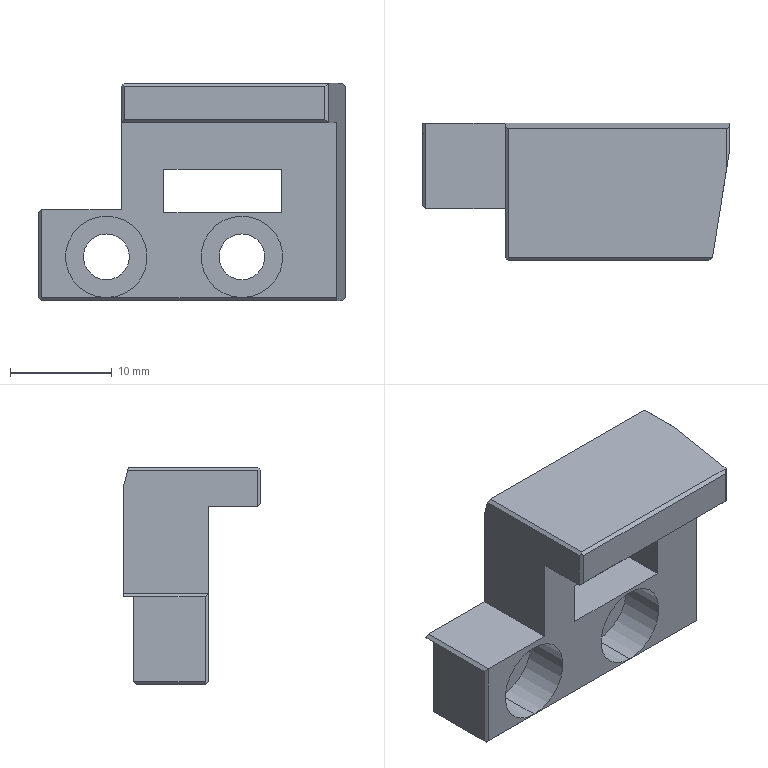Part | NX | 1 solid | 41 faces | box 30.1 x 13.5 x 21.378 mm | volume 3668 mm3 | plane 33 | cylinder 8 | commonest cylinder face diameters 4.5 x4 8 x4
STEP:
#1=CARTESIAN_POINT('',(-190.3,206.36,-59.));
#2=VERTEX_POINT('',#1);
#3=CARTESIAN_POINT('',(-219.8,206.36,-59.));
#4=VERTEX_POINT('',#3);
#5=CARTESIAN_POINT('',(-205.05,206.36,-59.));
#6=DIRECTION('',(-1.,0.,0.));
#7=VECTOR('',#6,1000.);
#8=LINE('',#5,#7);
#9=EDGE_CURVE('',#2,#4,#8,.T.);
#10=ORIENTED_EDGE('',*,*,#9,.F.);
#11=CARTESIAN_POINT('',(-190.3,202.995,-59.));
#12=VERTEX_POINT('',#11);
#13=CARTESIAN_POINT('',(-190.3,205.774,-59.));
#14=DIRECTION('',(0.,-1.,0.));
#15=VECTOR('',#14,1000.);
#16=LINE('',#13,#15);
#17=EDGE_CURVE('',#2,#12,#16,.T.);
#18=ORIENTED_EDGE('',*,*,#17,.T.);
#19=CARTESIAN_POINT('',(-190.838,199.6,-59.));
#20=VERTEX_POINT('',#19);
#21=CARTESIAN_POINT('',(-190.024,204.737,-59.));
#22=DIRECTION('',(0.1564,0.9877,0.));
#23=VECTOR('',#22,1000.);
#24=LINE('',#21,#23);
#25=EDGE_CURVE('',#20,#12,#24,.T.);
#26=ORIENTED_EDGE('',*,*,#25,.F.);
#27=CARTESIAN_POINT('',(-219.8,199.6,-59.));
#28=VERTEX_POINT('',#27);
#29=CARTESIAN_POINT('',(-205.493,199.6,-59.));
#30=DIRECTION('',(-1.,0.,0.));
#31=VECTOR('',#30,1000.);
#32=LINE('',#29,#31);
#33=EDGE_CURVE('',#20,#28,#32,.T.);
#34=ORIENTED_EDGE('',*,*,#33,.T.);
#35=CARTESIAN_POINT('',(-219.8,202.98,-59.));
#36=DIRECTION('',(0.,1.,0.));
#37=VECTOR('',#36,1000.);
#38=LINE('',#35,#37);
#39=EDGE_CURVE('',#28,#4,#38,.T.);
#40=ORIENTED_EDGE('',*,*,#39,.T.);
#41=EDGE_LOOP('',(#10,#18,#26,#34,#40));
#42=FACE_BOUND('',#41,.T.);
#43=CARTESIAN_POINT('',(-190.,199.3,-59.));
#44=DIRECTION('',(0.,0.,-1.));
#45=DIRECTION('',(0.,-1.,0.));
#46=AXIS2_PLACEMENT_3D('',#43,#44,#45);
#47=PLANE('',#46);
#48=ADVANCED_FACE('',(#42),#47,.T.);
#49=CARTESIAN_POINT('',(-211.7,194.16,-41.2));
#50=VERTEX_POINT('',#49);
#51=CARTESIAN_POINT('',(-191.999,194.16,-41.2));
#52=VERTEX_POINT('',#51);
#53=CARTESIAN_POINT('',(-201.85,194.16,-41.2));
#54=DIRECTION('',(1.,0.,0.));
#55=VECTOR('',#54,1000.);
#56=LINE('',#53,#55);
#57=EDGE_CURVE('',#50,#52,#56,.T.);
#58=ORIENTED_EDGE('',*,*,#57,.T.);
#59=CARTESIAN_POINT('',(-191.999,194.16,-37.922));
#60=VERTEX_POINT('',#59);
#61=CARTESIAN_POINT('',(-191.999,194.16,-39.561));
#62=DIRECTION('',(0.,0.,1.));
#63=VECTOR('',#62,1000.);
#64=LINE('',#61,#63);
#65=EDGE_CURVE('',#52,#60,#64,.T.);
#66=ORIENTED_EDGE('',*,*,#65,.T.);
#67=CARTESIAN_POINT('',(-211.7,194.16,-37.922));
#68=VERTEX_POINT('',#67);
#69=CARTESIAN_POINT('',(-201.85,194.16,-37.922));
#70=DIRECTION('',(1.,0.,0.));
#71=VECTOR('',#70,1000.);
#72=LINE('',#69,#71);
#73=EDGE_CURVE('',#68,#60,#72,.T.);
#74=ORIENTED_EDGE('',*,*,#73,.F.);
#75=CARTESIAN_POINT('',(-211.7,194.16,-39.561));
#76=DIRECTION('',(0.,0.,1.));
#77=VECTOR('',#76,1000.);
#78=LINE('',#75,#77);
#79=EDGE_CURVE('',#50,#68,#78,.T.);
#80=ORIENTED_EDGE('',*,*,#79,.F.);
#81=EDGE_LOOP('',(#58,#66,#74,#80));
#82=FACE_BOUND('',#81,.T.);
#83=CARTESIAN_POINT('',(-190.,194.16,-37.622));
#84=DIRECTION('',(0.,-1.,0.));
#85=DIRECTION('',(-1.,0.,0.));
#86=AXIS2_PLACEMENT_3D('',#83,#84,#85);
#87=PLANE('',#86);
#88=ADVANCED_FACE('',(#82),#87,.T.);
#89=CARTESIAN_POINT('',(-190.3,207.16,-37.622));
#90=VERTEX_POINT('',#89);
#91=CARTESIAN_POINT('',(-211.7,207.16,-37.622));
#92=VERTEX_POINT('',#91);
#93=CARTESIAN_POINT('',(-201.,207.16,-37.622));
#94=DIRECTION('',(-1.,0.,0.));
#95=VECTOR('',#94,1000.);
#96=LINE('',#93,#95);
#97=EDGE_CURVE('',#90,#92,#96,.T.);
#98=ORIENTED_EDGE('',*,*,#97,.T.);
#99=CARTESIAN_POINT('',(-211.7,194.46,-37.622));
#100=VERTEX_POINT('',#99);
#101=CARTESIAN_POINT('',(-211.7,204.737,-37.622));
#102=DIRECTION('',(0.,1.,0.));
#103=VECTOR('',#102,1000.);
#104=LINE('',#101,#103);
#105=EDGE_CURVE('',#100,#92,#104,.T.);
#106=ORIENTED_EDGE('',*,*,#105,.F.);
#107=CARTESIAN_POINT('',(-191.652,194.46,-37.622));
#108=VERTEX_POINT('',#107);
#109=CARTESIAN_POINT('',(-201.85,194.46,-37.622));
#110=DIRECTION('',(1.,0.,0.));
#111=VECTOR('',#110,1000.);
#112=LINE('',#109,#111);
#113=EDGE_CURVE('',#100,#108,#112,.T.);
#114=ORIENTED_EDGE('',*,*,#113,.T.);
#115=CARTESIAN_POINT('',(-190.3,202.995,-37.622));
#116=VERTEX_POINT('',#115);
#117=CARTESIAN_POINT('',(-190.024,204.737,-37.622));
#118=DIRECTION('',(-0.1564,-0.9877,0.));
#119=VECTOR('',#118,1000.);
#120=LINE('',#117,#119);
#121=EDGE_CURVE('',#116,#108,#120,.T.);
#122=ORIENTED_EDGE('',*,*,#121,.F.);
#123=CARTESIAN_POINT('',(-190.3,206.274,-37.622));
#124=DIRECTION('',(0.,-1.,0.));
#125=VECTOR('',#124,1000.);
#126=LINE('',#123,#125);
#127=EDGE_CURVE('',#90,#116,#126,.T.);
#128=ORIENTED_EDGE('',*,*,#127,.F.);
#129=EDGE_LOOP('',(#98,#106,#114,#122,#128));
#130=FACE_BOUND('',#129,.T.);
#131=CARTESIAN_POINT('',(-190.,207.9,-37.622));
#132=DIRECTION('',(0.,0.,1.));
#133=DIRECTION('',(1.,0.,0.));
#134=AXIS2_PLACEMENT_3D('',#131,#132,#133);
#135=PLANE('',#134);
#136=ADVANCED_FACE('',(#130),#135,.T.);
#137=CARTESIAN_POINT('',(-196.3,206.66,-50.35));
#138=VERTEX_POINT('',#137);
#139=CARTESIAN_POINT('',(-196.3,199.3,-50.35));
#140=VERTEX_POINT('',#139);
#141=CARTESIAN_POINT('',(-196.3,204.737,-50.35));
#142=DIRECTION('',(0.,-1.,0.));
#143=VECTOR('',#142,1000.);
#144=LINE('',#141,#143);
#145=EDGE_CURVE('',#138,#140,#144,.T.);
#146=ORIENTED_EDGE('',*,*,#145,.F.);
#147=CARTESIAN_POINT('',(-207.8,206.66,-50.35));
#148=VERTEX_POINT('',#147);
#149=CARTESIAN_POINT('',(-190.,206.66,-50.35));
#150=DIRECTION('',(-1.,0.,0.));
#151=VECTOR('',#150,1000.);
#152=LINE('',#149,#151);
#153=EDGE_CURVE('',#138,#148,#152,.T.);
#154=ORIENTED_EDGE('',*,*,#153,.T.);
#155=CARTESIAN_POINT('',(-207.8,199.3,-50.35));
#156=VERTEX_POINT('',#155);
#157=CARTESIAN_POINT('',(-207.8,204.737,-50.35));
#158=DIRECTION('',(0.,1.,0.));
#159=VECTOR('',#158,1000.);
#160=LINE('',#157,#159);
#161=EDGE_CURVE('',#156,#148,#160,.T.);
#162=ORIENTED_EDGE('',*,*,#161,.F.);
#163=CARTESIAN_POINT('',(-190.,199.3,-50.35));
#164=DIRECTION('',(-1.,0.,0.));
#165=VECTOR('',#164,1000.);
#166=LINE('',#163,#165);
#167=EDGE_CURVE('',#140,#156,#166,.T.);
#168=ORIENTED_EDGE('',*,*,#167,.F.);
#169=EDGE_LOOP('',(#146,#154,#162,#168));
#170=FACE_BOUND('',#169,.T.);
#171=CARTESIAN_POINT('',(-206.8,198.44,-50.35));
#172=DIRECTION('',(0.,0.,-1.));
#173=DIRECTION('',(0.,-1.,0.));
#174=AXIS2_PLACEMENT_3D('',#171,#172,#173);
#175=PLANE('',#174);
#176=ADVANCED_FACE('',(#170),#175,.F.);
#177=CARTESIAN_POINT('',(-212.,207.66,-50.05));
#178=VERTEX_POINT('',#177);
#179=CARTESIAN_POINT('',(-219.8,207.66,-50.05));
#180=VERTEX_POINT('',#179);
#181=CARTESIAN_POINT('',(-190.,207.66,-50.05));
#182=DIRECTION('',(-1.,0.,0.));
#183=VECTOR('',#182,1000.);
#184=LINE('',#181,#183);
#185=EDGE_CURVE('',#178,#180,#184,.T.);
#186=ORIENTED_EDGE('',*,*,#185,.T.);
#187=CARTESIAN_POINT('',(-219.8,199.3,-50.05));
#188=VERTEX_POINT('',#187);
#189=CARTESIAN_POINT('',(-219.8,203.48,-50.05));
#190=DIRECTION('',(0.,-1.,0.));
#191=VECTOR('',#190,1000.);
#192=LINE('',#189,#191);
#193=EDGE_CURVE('',#180,#188,#192,.T.);
#194=ORIENTED_EDGE('',*,*,#193,.T.);
#195=CARTESIAN_POINT('',(-212.,199.3,-50.05));
#196=VERTEX_POINT('',#195);
#197=CARTESIAN_POINT('',(-190.,199.3,-50.05));
#198=DIRECTION('',(1.,0.,0.));
#199=VECTOR('',#198,1000.);
#200=LINE('',#197,#199);
#201=EDGE_CURVE('',#188,#196,#200,.T.);
#202=ORIENTED_EDGE('',*,*,#201,.T.);
#203=CARTESIAN_POINT('',(-212.,204.737,-50.05));
#204=DIRECTION('',(0.,-1.,0.));
#205=VECTOR('',#204,1000.);
#206=LINE('',#203,#205);
#207=EDGE_CURVE('',#178,#196,#206,.T.);
#208=ORIENTED_EDGE('',*,*,#207,.F.);
#209=EDGE_LOOP('',(#186,#194,#202,#208));
#210=FACE_BOUND('',#209,.T.);
#211=CARTESIAN_POINT('',(-216.1,198.44,-50.05));
#212=DIRECTION('',(0.,0.,-1.));
#213=DIRECTION('',(0.,-1.,0.));
#214=AXIS2_PLACEMENT_3D('',#211,#212,#213);
#215=PLANE('',#214);
#216=ADVANCED_FACE('',(#210),#215,.F.);
#217=CARTESIAN_POINT('',(-212.,194.46,-41.5));
#218=VERTEX_POINT('',#217);
#219=CARTESIAN_POINT('',(-212.,194.46,-37.922));
#220=VERTEX_POINT('',#219);
#221=CARTESIAN_POINT('',(-212.,194.46,-39.561));
#222=DIRECTION('',(0.,0.,1.));
#223=VECTOR('',#222,1000.);
#224=LINE('',#221,#223);
#225=EDGE_CURVE('',#218,#220,#224,.T.);
#226=ORIENTED_EDGE('',*,*,#225,.T.);
#227=CARTESIAN_POINT('',(-212.,207.235,-37.922));
#228=VERTEX_POINT('',#227);
#229=CARTESIAN_POINT('',(-212.,204.737,-37.922));
#230=DIRECTION('',(0.,1.,0.));
#231=VECTOR('',#230,1000.);
#232=LINE('',#229,#231);
#233=EDGE_CURVE('',#220,#228,#232,.T.);
#234=ORIENTED_EDGE('',*,*,#233,.T.);
#235=CARTESIAN_POINT('',(-212.,207.66,-39.622));
#236=VERTEX_POINT('',#235);
#237=CARTESIAN_POINT('',(-212.,208.682,-43.71));
#238=DIRECTION('',(0.,0.2425,-0.9701));
#239=VECTOR('',#238,1000.);
#240=LINE('',#237,#239);
#241=EDGE_CURVE('',#228,#236,#240,.T.);
#242=ORIENTED_EDGE('',*,*,#241,.T.);
#243=CARTESIAN_POINT('',(-212.,207.66,-43.71));
#244=DIRECTION('',(0.,0.,1.));
#245=VECTOR('',#244,1000.);
#246=LINE('',#243,#245);
#247=EDGE_CURVE('',#178,#236,#246,.T.);
#248=ORIENTED_EDGE('',*,*,#247,.F.);
#249=ORIENTED_EDGE('',*,*,#207,.T.);
#250=CARTESIAN_POINT('',(-212.,199.3,-41.5));
#251=VERTEX_POINT('',#250);
#252=CARTESIAN_POINT('',(-212.,199.3,-43.71));
#253=DIRECTION('',(0.,0.,1.));
#254=VECTOR('',#253,1000.);
#255=LINE('',#252,#254);
#256=EDGE_CURVE('',#196,#251,#255,.T.);
#257=ORIENTED_EDGE('',*,*,#256,.T.);
#258=CARTESIAN_POINT('',(-212.,204.737,-41.5));
#259=DIRECTION('',(0.,1.,0.));
#260=VECTOR('',#259,1000.);
#261=LINE('',#258,#260);
#262=EDGE_CURVE('',#218,#251,#261,.T.);
#263=ORIENTED_EDGE('',*,*,#262,.F.);
#264=EDGE_LOOP('',(#226,#234,#242,#248,#249,#257,#263));
#265=FACE_BOUND('',#264,.T.);
#266=CARTESIAN_POINT('',(-212.,198.44,-46.8));
#267=DIRECTION('',(1.,0.,0.));
#268=DIRECTION('',(0.,-1.,0.));
#269=AXIS2_PLACEMENT_3D('',#266,#267,#268);
#270=PLANE('',#269);
#271=ADVANCED_FACE('',(#265),#270,.F.);
#272=ORIENTED_EDGE('',*,*,#225,.F.);
#273=CARTESIAN_POINT('',(-190.,172.46,-19.5));
#274=DIRECTION('',(0.5774,-0.5774,0.5774));
#275=VECTOR('',#274,1000.);
#276=LINE('',#273,#275);
#277=EDGE_CURVE('',#218,#50,#276,.T.);
#278=ORIENTED_EDGE('',*,*,#277,.T.);
#279=ORIENTED_EDGE('',*,*,#79,.T.);
#280=CARTESIAN_POINT('',(-211.85,194.31,-37.772));
#281=VERTEX_POINT('',#280);
#282=CARTESIAN_POINT('',(-190.,172.46,-59.622));
#283=DIRECTION('',(0.5774,-0.5774,-0.5774));
#284=VECTOR('',#283,1000.);
#285=LINE('',#282,#284);
#286=EDGE_CURVE('',#281,#68,#285,.T.);
#287=ORIENTED_EDGE('',*,*,#286,.F.);
#288=CARTESIAN_POINT('',(-190.,172.46,-15.922));
#289=DIRECTION('',(0.5774,-0.5774,0.5774));
#290=VECTOR('',#289,1000.);
#291=LINE('',#288,#290);
#292=EDGE_CURVE('',#220,#281,#291,.T.);
#293=ORIENTED_EDGE('',*,*,#292,.F.);
#294=EDGE_LOOP('',(#272,#278,#279,#287,#293));
#295=FACE_BOUND('',#294,.T.);
#296=CARTESIAN_POINT('',(-211.85,194.31,-39.561));
#297=DIRECTION('',(-0.7071,-0.7071,0.));
#298=DIRECTION('',(-0.7071,0.7071,0.));
#299=AXIS2_PLACEMENT_3D('',#296,#297,#298);
#300=PLANE('',#299);
#301=ADVANCED_FACE('',(#295),#300,.T.);
#302=CARTESIAN_POINT('',(-196.3,207.66,-50.35));
#303=VERTEX_POINT('',#302);
#304=CARTESIAN_POINT('',(-196.3,204.737,-50.35));
#305=DIRECTION('',(0.,1.,0.));
#306=VECTOR('',#305,1000.);
#307=LINE('',#304,#306);
#308=EDGE_CURVE('',#138,#303,#307,.T.);
#309=ORIENTED_EDGE('',*,*,#308,.F.);
#310=ORIENTED_EDGE('',*,*,#145,.T.);
#311=CARTESIAN_POINT('',(-196.3,199.3,-46.1));
#312=VERTEX_POINT('',#311);
#313=CARTESIAN_POINT('',(-196.3,199.3,-43.71));
#314=DIRECTION('',(0.,0.,1.));
#315=VECTOR('',#314,1000.);
#316=LINE('',#313,#315);
#317=EDGE_CURVE('',#140,#312,#316,.T.);
#318=ORIENTED_EDGE('',*,*,#317,.T.);
#319=CARTESIAN_POINT('',(-196.3,207.66,-46.1));
#320=VERTEX_POINT('',#319);
#321=CARTESIAN_POINT('',(-196.3,204.737,-46.1));
#322=DIRECTION('',(0.,1.,0.));
#323=VECTOR('',#322,1000.);
#324=LINE('',#321,#323);
#325=EDGE_CURVE('',#312,#320,#324,.T.);
#326=ORIENTED_EDGE('',*,*,#325,.T.);
#327=CARTESIAN_POINT('',(-196.3,207.66,-43.71));
#328=DIRECTION('',(0.,0.,-1.));
#329=VECTOR('',#328,1000.);
#330=LINE('',#327,#329);
#331=EDGE_CURVE('',#320,#303,#330,.T.);
#332=ORIENTED_EDGE('',*,*,#331,.T.);
#333=EDGE_LOOP('',(#309,#310,#318,#326,#332));
#334=FACE_BOUND('',#333,.T.);
#335=CARTESIAN_POINT('',(-196.3,198.44,-50.35));
#336=DIRECTION('',(1.,0.,0.));
#337=DIRECTION('',(0.,-1.,0.));
#338=AXIS2_PLACEMENT_3D('',#335,#336,#337);
#339=PLANE('',#338);
#340=ADVANCED_FACE('',(#334),#339,.F.);
#341=CARTESIAN_POINT('',(-207.8,199.3,-46.1));
#342=VERTEX_POINT('',#341);
#343=CARTESIAN_POINT('',(-207.8,199.3,-43.71));
#344=DIRECTION('',(0.,0.,1.));
#345=VECTOR('',#344,1000.);
#346=LINE('',#343,#345);
#347=EDGE_CURVE('',#156,#342,#346,.T.);
#348=ORIENTED_EDGE('',*,*,#347,.F.);
#349=ORIENTED_EDGE('',*,*,#161,.T.);
#350=CARTESIAN_POINT('',(-207.8,207.66,-50.35));
#351=VERTEX_POINT('',#350);
#352=CARTESIAN_POINT('',(-207.8,204.737,-50.35));
#353=DIRECTION('',(0.,1.,0.));
#354=VECTOR('',#353,1000.);
#355=LINE('',#352,#354);
#356=EDGE_CURVE('',#148,#351,#355,.T.);
#357=ORIENTED_EDGE('',*,*,#356,.T.);
#358=CARTESIAN_POINT('',(-207.8,207.66,-46.1));
#359=VERTEX_POINT('',#358);
#360=CARTESIAN_POINT('',(-207.8,207.66,-43.71));
#361=DIRECTION('',(0.,0.,1.));
#362=VECTOR('',#361,1000.);
#363=LINE('',#360,#362);
#364=EDGE_CURVE('',#351,#359,#363,.T.);
#365=ORIENTED_EDGE('',*,*,#364,.T.);
#366=CARTESIAN_POINT('',(-207.8,204.737,-46.1));
#367=DIRECTION('',(0.,1.,0.));
#368=VECTOR('',#367,1000.);
#369=LINE('',#366,#368);
#370=EDGE_CURVE('',#342,#359,#369,.T.);
#371=ORIENTED_EDGE('',*,*,#370,.F.);
#372=EDGE_LOOP('',(#348,#349,#357,#365,#371));
#373=FACE_BOUND('',#372,.T.);
#374=CARTESIAN_POINT('',(-207.8,198.44,-47.1));
#375=DIRECTION('',(-1.,0.,0.));
#376=DIRECTION('',(0.,0.,1.));
#377=AXIS2_PLACEMENT_3D('',#374,#375,#376);
#378=PLANE('',#377);
#379=ADVANCED_FACE('',(#373),#378,.F.);
#380=ORIENTED_EDGE('',*,*,#247,.T.);
#381=CARTESIAN_POINT('',(-190.,207.66,-39.622));
#382=VERTEX_POINT('',#381);
#383=CARTESIAN_POINT('',(-201.,207.66,-39.622));
#384=DIRECTION('',(-1.,0.,0.));
#385=VECTOR('',#384,1000.);
#386=LINE('',#383,#385);
#387=EDGE_CURVE('',#382,#236,#386,.T.);
#388=ORIENTED_EDGE('',*,*,#387,.F.);
#389=CARTESIAN_POINT('',(-190.,207.66,-50.35));
#390=VERTEX_POINT('',#389);
#391=CARTESIAN_POINT('',(-190.,207.66,-43.71));
#392=DIRECTION('',(0.,0.,-1.));
#393=VECTOR('',#392,1000.);
#394=LINE('',#391,#393);
#395=EDGE_CURVE('',#382,#390,#394,.T.);
#396=ORIENTED_EDGE('',*,*,#395,.T.);
#397=CARTESIAN_POINT('',(-190.,207.66,-50.35));
#398=DIRECTION('',(1.,0.,0.));
#399=VECTOR('',#398,1000.);
#400=LINE('',#397,#399);
#401=EDGE_CURVE('',#303,#390,#400,.T.);
#402=ORIENTED_EDGE('',*,*,#401,.F.);
#403=ORIENTED_EDGE('',*,*,#331,.F.);
#404=CARTESIAN_POINT('',(-190.,207.66,-46.1));
#405=DIRECTION('',(-1.,0.,0.));
#406=VECTOR('',#405,1000.);
#407=LINE('',#404,#406);
#408=EDGE_CURVE('',#320,#359,#407,.T.);
#409=ORIENTED_EDGE('',*,*,#408,.T.);
#410=ORIENTED_EDGE('',*,*,#364,.F.);
#411=CARTESIAN_POINT('',(-220.1,207.66,-50.35));
#412=VERTEX_POINT('',#411);
#413=CARTESIAN_POINT('',(-190.,207.66,-50.35));
#414=DIRECTION('',(1.,0.,0.));
#415=VECTOR('',#414,1000.);
#416=LINE('',#413,#415);
#417=EDGE_CURVE('',#412,#351,#416,.T.);
#418=ORIENTED_EDGE('',*,*,#417,.F.);
#419=CARTESIAN_POINT('',(-190.,207.66,-20.25));
#420=DIRECTION('',(0.7071,0.,0.7071));
#421=VECTOR('',#420,1000.);
#422=LINE('',#419,#421);
#423=EDGE_CURVE('',#412,#180,#422,.T.);
#424=ORIENTED_EDGE('',*,*,#423,.T.);
#425=ORIENTED_EDGE('',*,*,#185,.F.);
#426=EDGE_LOOP('',(#380,#388,#396,#402,#403,#409,#410,#418,#424,#425));
#427=FACE_BOUND('',#426,.T.);
#428=CARTESIAN_POINT('',(-190.,207.66,-59.));
#429=DIRECTION('',(0.,1.,0.));
#430=DIRECTION('',(1.,0.,0.));
#431=AXIS2_PLACEMENT_3D('',#428,#429,#430);
#432=PLANE('',#431);
#433=ADVANCED_FACE('',(#427),#432,.T.);
#434=ORIENTED_EDGE('',*,*,#308,.T.);
#435=ORIENTED_EDGE('',*,*,#401,.T.);
#436=CARTESIAN_POINT('',(-190.,206.66,-50.35));
#437=VERTEX_POINT('',#436);
#438=CARTESIAN_POINT('',(-190.,204.737,-50.35));
#439=DIRECTION('',(0.,1.,0.));
#440=VECTOR('',#439,1000.);
#441=LINE('',#438,#440);
#442=EDGE_CURVE('',#437,#390,#441,.T.);
#443=ORIENTED_EDGE('',*,*,#442,.F.);
#444=CARTESIAN_POINT('',(-186.99,206.66,-50.35));
#445=DIRECTION('',(-1.,0.,0.));
#446=VECTOR('',#445,1000.);
#447=LINE('',#444,#446);
#448=EDGE_CURVE('',#437,#138,#447,.T.);
#449=ORIENTED_EDGE('',*,*,#448,.T.);
#450=EDGE_LOOP('',(#434,#435,#443,#449));
#451=FACE_BOUND('',#450,.T.);
#452=CARTESIAN_POINT('',(-186.99,249.9,-50.35));
#453=DIRECTION('',(0.,0.,1.));
#454=DIRECTION('',(1.,0.,0.));
#455=AXIS2_PLACEMENT_3D('',#452,#453,#454);
#456=PLANE('',#455);
#457=ADVANCED_FACE('',(#451),#456,.F.);
#458=ORIENTED_EDGE('',*,*,#417,.T.);
#459=ORIENTED_EDGE('',*,*,#356,.F.);
#460=CARTESIAN_POINT('',(-220.1,206.66,-50.35));
#461=VERTEX_POINT('',#460);
#462=CARTESIAN_POINT('',(-186.99,206.66,-50.35));
#463=DIRECTION('',(-1.,0.,0.));
#464=VECTOR('',#463,1000.);
#465=LINE('',#462,#464);
#466=EDGE_CURVE('',#148,#461,#465,.T.);
#467=ORIENTED_EDGE('',*,*,#466,.T.);
#468=CARTESIAN_POINT('',(-220.1,203.48,-50.35));
#469=DIRECTION('',(0.,-1.,0.));
#470=VECTOR('',#469,1000.);
#471=LINE('',#468,#470);
#472=EDGE_CURVE('',#412,#461,#471,.T.);
#473=ORIENTED_EDGE('',*,*,#472,.F.);
#474=EDGE_LOOP('',(#458,#459,#467,#473));
#475=FACE_BOUND('',#474,.T.);
#476=CARTESIAN_POINT('',(-186.99,249.9,-50.35));
#477=DIRECTION('',(0.,0.,1.));
#478=DIRECTION('',(1.,0.,0.));
#479=AXIS2_PLACEMENT_3D('',#476,#477,#478);
#480=PLANE('',#479);
#481=ADVANCED_FACE('',(#475),#480,.F.);
#482=ORIENTED_EDGE('',*,*,#448,.F.);
#483=CARTESIAN_POINT('',(-190.,206.66,-58.7));
#484=VERTEX_POINT('',#483);
#485=CARTESIAN_POINT('',(-190.,206.66,-43.71));
#486=DIRECTION('',(0.,0.,1.));
#487=VECTOR('',#486,1000.);
#488=LINE('',#485,#487);
#489=EDGE_CURVE('',#484,#437,#488,.T.);
#490=ORIENTED_EDGE('',*,*,#489,.F.);
#491=CARTESIAN_POINT('',(-220.1,206.66,-58.7));
#492=VERTEX_POINT('',#491);
#493=CARTESIAN_POINT('',(-205.05,206.66,-58.7));
#494=DIRECTION('',(-1.,0.,0.));
#495=VECTOR('',#494,1000.);
#496=LINE('',#493,#495);
#497=EDGE_CURVE('',#484,#492,#496,.T.);
#498=ORIENTED_EDGE('',*,*,#497,.T.);
#499=CARTESIAN_POINT('',(-220.1,206.66,-43.71));
#500=DIRECTION('',(0.,0.,1.));
#501=VECTOR('',#500,1000.);
#502=LINE('',#499,#501);
#503=EDGE_CURVE('',#492,#461,#502,.T.);
#504=ORIENTED_EDGE('',*,*,#503,.T.);
#505=ORIENTED_EDGE('',*,*,#466,.F.);
#506=ORIENTED_EDGE('',*,*,#153,.F.);
#507=EDGE_LOOP('',(#482,#490,#498,#504,#505,#506));
#508=FACE_BOUND('',#507,.T.);
#509=CARTESIAN_POINT('',(-200.15,206.66,-52.425));
#510=VERTEX_POINT('',#509);
#511=CARTESIAN_POINT('',(-200.15,206.66,-56.925));
#512=VERTEX_POINT('',#511);
#513=CARTESIAN_POINT('',(-200.15,206.66,-54.675));
#514=DIRECTION('',(0.,-1.,0.));
#515=DIRECTION('',(0.,0.,-1.));
#516=AXIS2_PLACEMENT_3D('',#513,#514,#515);
#517=CIRCLE('',#516,2.25);
#518=EDGE_CURVE('',#510,#512,#517,.T.);
#519=ORIENTED_EDGE('',*,*,#518,.T.);
#520=CARTESIAN_POINT('',(-200.15,206.66,-54.675));
#521=DIRECTION('',(0.,-1.,0.));
#522=DIRECTION('',(0.,0.,-1.));
#523=AXIS2_PLACEMENT_3D('',#520,#521,#522);
#524=CIRCLE('',#523,2.25);
#525=EDGE_CURVE('',#512,#510,#524,.T.);
#526=ORIENTED_EDGE('',*,*,#525,.T.);
#527=EDGE_LOOP('',(#519,#526));
#528=FACE_BOUND('',#527,.T.);
#529=CARTESIAN_POINT('',(-213.45,206.66,-52.425));
#530=VERTEX_POINT('',#529);
#531=CARTESIAN_POINT('',(-213.45,206.66,-56.925));
#532=VERTEX_POINT('',#531);
#533=CARTESIAN_POINT('',(-213.45,206.66,-54.675));
#534=DIRECTION('',(0.,-1.,0.));
#535=DIRECTION('',(0.,0.,-1.));
#536=AXIS2_PLACEMENT_3D('',#533,#534,#535);
#537=CIRCLE('',#536,2.25);
#538=EDGE_CURVE('',#530,#532,#537,.T.);
#539=ORIENTED_EDGE('',*,*,#538,.T.);
#540=CARTESIAN_POINT('',(-213.45,206.66,-54.675));
#541=DIRECTION('',(0.,-1.,0.));
#542=DIRECTION('',(0.,0.,-1.));
#543=AXIS2_PLACEMENT_3D('',#540,#541,#542);
#544=CIRCLE('',#543,2.25);
#545=EDGE_CURVE('',#532,#530,#544,.T.);
#546=ORIENTED_EDGE('',*,*,#545,.T.);
#547=EDGE_LOOP('',(#539,#546));
#548=FACE_BOUND('',#547,.T.);
#549=CARTESIAN_POINT('',(-186.99,206.66,-50.35));
#550=DIRECTION('',(0.,-1.,0.));
#551=DIRECTION('',(-1.,0.,0.));
#552=AXIS2_PLACEMENT_3D('',#549,#550,#551);
#553=PLANE('',#552);
#554=ADVANCED_FACE('',(#508,#528,#548),#553,.F.);
#555=CARTESIAN_POINT('',(-213.45,199.3,-50.675));
#556=VERTEX_POINT('',#555);
#557=CARTESIAN_POINT('',(-213.45,199.3,-58.675));
#558=VERTEX_POINT('',#557);
#559=CARTESIAN_POINT('',(-213.45,199.3,-54.675));
#560=DIRECTION('',(0.,-1.,0.));
#561=DIRECTION('',(0.,0.,-1.));
#562=AXIS2_PLACEMENT_3D('',#559,#560,#561);
#563=CIRCLE('',#562,4.);
#564=EDGE_CURVE('',#556,#558,#563,.T.);
#565=ORIENTED_EDGE('',*,*,#564,.T.);
#566=CARTESIAN_POINT('',(-213.45,203.8,-58.675));
#567=VERTEX_POINT('',#566);
#568=CARTESIAN_POINT('',(-213.45,194.3,-58.675));
#569=DIRECTION('',(0.,-1.,0.));
#570=VECTOR('',#569,1000.);
#571=LINE('',#568,#570);
#572=EDGE_CURVE('',#558,#567,#571,.F.);
#573=ORIENTED_EDGE('',*,*,#572,.T.);
#574=CARTESIAN_POINT('',(-213.45,203.8,-50.675));
#575=VERTEX_POINT('',#574);
#576=CARTESIAN_POINT('',(-213.45,203.8,-54.675));
#577=DIRECTION('',(0.,-1.,0.));
#578=DIRECTION('',(0.,0.,-1.));
#579=AXIS2_PLACEMENT_3D('',#576,#577,#578);
#580=CIRCLE('',#579,4.);
#581=EDGE_CURVE('',#575,#567,#580,.T.);
#582=ORIENTED_EDGE('',*,*,#581,.F.);
#583=CARTESIAN_POINT('',(-213.45,194.3,-50.675));
#584=DIRECTION('',(0.,-1.,0.));
#585=VECTOR('',#584,1000.);
#586=LINE('',#583,#585);
#587=EDGE_CURVE('',#556,#575,#586,.F.);
#588=ORIENTED_EDGE('',*,*,#587,.F.);
#589=EDGE_LOOP('',(#565,#573,#582,#588));
#590=FACE_BOUND('',#589,.T.);
#591=CARTESIAN_POINT('',(-213.45,194.3,-54.675));
#592=DIRECTION('',(0.,-1.,0.));
#593=DIRECTION('',(0.,0.,-1.));
#594=AXIS2_PLACEMENT_3D('',#591,#592,#593);
#595=CYLINDRICAL_SURFACE('',#594,4.);
#596=ADVANCED_FACE('',(#590),#595,.F.);
#597=ORIENTED_EDGE('',*,*,#581,.T.);
#598=CARTESIAN_POINT('',(-213.45,203.8,-54.675));
#599=DIRECTION('',(0.,-1.,0.));
#600=DIRECTION('',(0.,0.,-1.));
#601=AXIS2_PLACEMENT_3D('',#598,#599,#600);
#602=CIRCLE('',#601,4.);
#603=EDGE_CURVE('',#567,#575,#602,.T.);
#604=ORIENTED_EDGE('',*,*,#603,.T.);
#605=EDGE_LOOP('',(#597,#604));
#606=FACE_BOUND('',#605,.T.);
#607=CARTESIAN_POINT('',(-213.45,203.8,-52.425));
#608=VERTEX_POINT('',#607);
#609=CARTESIAN_POINT('',(-213.45,203.8,-56.925));
#610=VERTEX_POINT('',#609);
#611=CARTESIAN_POINT('',(-213.45,203.8,-54.675));
#612=DIRECTION('',(0.,-1.,0.));
#613=DIRECTION('',(0.,0.,-1.));
#614=AXIS2_PLACEMENT_3D('',#611,#612,#613);
#615=CIRCLE('',#614,2.25);
#616=EDGE_CURVE('',#608,#610,#615,.T.);
#617=ORIENTED_EDGE('',*,*,#616,.F.);
#618=CARTESIAN_POINT('',(-213.45,203.8,-54.675));
#619=DIRECTION('',(0.,-1.,0.));
#620=DIRECTION('',(0.,0.,-1.));
#621=AXIS2_PLACEMENT_3D('',#618,#619,#620);
#622=CIRCLE('',#621,2.25);
#623=EDGE_CURVE('',#610,#608,#622,.T.);
#624=ORIENTED_EDGE('',*,*,#623,.F.);
#625=EDGE_LOOP('',(#617,#624));
#626=FACE_BOUND('',#625,.T.);
#627=CARTESIAN_POINT('',(-213.45,203.8,-54.675));
#628=DIRECTION('',(0.,-1.,0.));
#629=DIRECTION('',(-1.,0.,0.));
#630=AXIS2_PLACEMENT_3D('',#627,#628,#629);
#631=PLANE('',#630);
#632=ADVANCED_FACE('',(#606,#626),#631,.T.);
#633=ORIENTED_EDGE('',*,*,#616,.T.);
#634=CARTESIAN_POINT('',(-213.45,194.3,-56.925));
#635=DIRECTION('',(0.,-1.,0.));
#636=VECTOR('',#635,1000.);
#637=LINE('',#634,#636);
#638=EDGE_CURVE('',#532,#610,#637,.T.);
#639=ORIENTED_EDGE('',*,*,#638,.F.);
#640=ORIENTED_EDGE('',*,*,#538,.F.);
#641=CARTESIAN_POINT('',(-213.45,194.3,-52.425));
#642=DIRECTION('',(0.,-1.,0.));
#643=VECTOR('',#642,1000.);
#644=LINE('',#641,#643);
#645=EDGE_CURVE('',#530,#608,#644,.T.);
#646=ORIENTED_EDGE('',*,*,#645,.T.);
#647=EDGE_LOOP('',(#633,#639,#640,#646));
#648=FACE_BOUND('',#647,.T.);
#649=CARTESIAN_POINT('',(-213.45,194.3,-54.675));
#650=DIRECTION('',(0.,-1.,0.));
#651=DIRECTION('',(0.,0.,-1.));
#652=AXIS2_PLACEMENT_3D('',#649,#650,#651);
#653=CYLINDRICAL_SURFACE('',#652,2.25);
#654=ADVANCED_FACE('',(#648),#653,.F.);
#655=CARTESIAN_POINT('',(-200.15,203.8,-52.425));
#656=VERTEX_POINT('',#655);
#657=CARTESIAN_POINT('',(-200.15,203.8,-56.925));
#658=VERTEX_POINT('',#657);
#659=CARTESIAN_POINT('',(-200.15,203.8,-54.675));
#660=DIRECTION('',(0.,-1.,0.));
#661=DIRECTION('',(0.,0.,-1.));
#662=AXIS2_PLACEMENT_3D('',#659,#660,#661);
#663=CIRCLE('',#662,2.25);
#664=EDGE_CURVE('',#656,#658,#663,.T.);
#665=ORIENTED_EDGE('',*,*,#664,.T.);
#666=CARTESIAN_POINT('',(-200.15,194.3,-56.925));
#667=DIRECTION('',(0.,-1.,0.));
#668=VECTOR('',#667,1000.);
#669=LINE('',#666,#668);
#670=EDGE_CURVE('',#512,#658,#669,.T.);
#671=ORIENTED_EDGE('',*,*,#670,.F.);
#672=ORIENTED_EDGE('',*,*,#518,.F.);
#673=CARTESIAN_POINT('',(-200.15,194.3,-52.425));
#674=DIRECTION('',(0.,-1.,0.));
#675=VECTOR('',#674,1000.);
#676=LINE('',#673,#675);
#677=EDGE_CURVE('',#510,#656,#676,.T.);
#678=ORIENTED_EDGE('',*,*,#677,.T.);
#679=EDGE_LOOP('',(#665,#671,#672,#678));
#680=FACE_BOUND('',#679,.T.);
#681=CARTESIAN_POINT('',(-200.15,194.3,-54.675));
#682=DIRECTION('',(0.,-1.,0.));
#683=DIRECTION('',(0.,0.,-1.));
#684=AXIS2_PLACEMENT_3D('',#681,#682,#683);
#685=CYLINDRICAL_SURFACE('',#684,2.25);
#686=ADVANCED_FACE('',(#680),#685,.F.);
#687=CARTESIAN_POINT('',(-200.15,203.8,-50.675));
#688=VERTEX_POINT('',#687);
#689=CARTESIAN_POINT('',(-200.15,203.8,-58.675));
#690=VERTEX_POINT('',#689);
#691=CARTESIAN_POINT('',(-200.15,203.8,-54.675));
#692=DIRECTION('',(0.,-1.,0.));
#693=DIRECTION('',(0.,0.,-1.));
#694=AXIS2_PLACEMENT_3D('',#691,#692,#693);
#695=CIRCLE('',#694,4.);
#696=EDGE_CURVE('',#688,#690,#695,.T.);
#697=ORIENTED_EDGE('',*,*,#696,.T.);
#698=CARTESIAN_POINT('',(-200.15,203.8,-54.675));
#699=DIRECTION('',(0.,-1.,0.));
#700=DIRECTION('',(0.,0.,-1.));
#701=AXIS2_PLACEMENT_3D('',#698,#699,#700);
#702=CIRCLE('',#701,4.);
#703=EDGE_CURVE('',#690,#688,#702,.T.);
#704=ORIENTED_EDGE('',*,*,#703,.T.);
#705=EDGE_LOOP('',(#697,#704));
#706=FACE_BOUND('',#705,.T.);
#707=ORIENTED_EDGE('',*,*,#664,.F.);
#708=CARTESIAN_POINT('',(-200.15,203.8,-54.675));
#709=DIRECTION('',(0.,-1.,0.));
#710=DIRECTION('',(0.,0.,-1.));
#711=AXIS2_PLACEMENT_3D('',#708,#709,#710);
#712=CIRCLE('',#711,2.25);
#713=EDGE_CURVE('',#658,#656,#712,.T.);
#714=ORIENTED_EDGE('',*,*,#713,.F.);
#715=EDGE_LOOP('',(#707,#714));
#716=FACE_BOUND('',#715,.T.);
#717=CARTESIAN_POINT('',(-200.15,203.8,-54.675));
#718=DIRECTION('',(0.,-1.,0.));
#719=DIRECTION('',(-1.,0.,0.));
#720=AXIS2_PLACEMENT_3D('',#717,#718,#719);
#721=PLANE('',#720);
#722=ADVANCED_FACE('',(#706,#716),#721,.T.);
#723=CARTESIAN_POINT('',(-200.15,199.3,-50.675));
#724=VERTEX_POINT('',#723);
#725=CARTESIAN_POINT('',(-200.15,199.3,-58.675));
#726=VERTEX_POINT('',#725);
#727=CARTESIAN_POINT('',(-200.15,199.3,-54.675));
#728=DIRECTION('',(0.,-1.,0.));
#729=DIRECTION('',(0.,0.,-1.));
#730=AXIS2_PLACEMENT_3D('',#727,#728,#729);
#731=CIRCLE('',#730,4.);
#732=EDGE_CURVE('',#724,#726,#731,.T.);
#733=ORIENTED_EDGE('',*,*,#732,.T.);
#734=CARTESIAN_POINT('',(-200.15,194.3,-58.675));
#735=DIRECTION('',(0.,-1.,0.));
#736=VECTOR('',#735,1000.);
#737=LINE('',#734,#736);
#738=EDGE_CURVE('',#726,#690,#737,.F.);
#739=ORIENTED_EDGE('',*,*,#738,.T.);
#740=ORIENTED_EDGE('',*,*,#696,.F.);
#741=CARTESIAN_POINT('',(-200.15,194.3,-50.675));
#742=DIRECTION('',(0.,-1.,0.));
#743=VECTOR('',#742,1000.);
#744=LINE('',#741,#743);
#745=EDGE_CURVE('',#724,#688,#744,.F.);
#746=ORIENTED_EDGE('',*,*,#745,.F.);
#747=EDGE_LOOP('',(#733,#739,#740,#746));
#748=FACE_BOUND('',#747,.T.);
#749=CARTESIAN_POINT('',(-200.15,194.3,-54.675));
#750=DIRECTION('',(0.,-1.,0.));
#751=DIRECTION('',(0.,0.,-1.));
#752=AXIS2_PLACEMENT_3D('',#749,#750,#751);
#753=CYLINDRICAL_SURFACE('',#752,4.);
#754=ADVANCED_FACE('',(#748),#753,.F.);
#755=CARTESIAN_POINT('',(-190.885,199.3,-58.7));
#756=VERTEX_POINT('',#755);
#757=CARTESIAN_POINT('',(-219.8,199.3,-58.7));
#758=VERTEX_POINT('',#757);
#759=CARTESIAN_POINT('',(-205.493,199.3,-58.7));
#760=DIRECTION('',(-1.,0.,0.));
#761=VECTOR('',#760,1000.);
#762=LINE('',#759,#761);
#763=EDGE_CURVE('',#756,#758,#762,.T.);
#764=ORIENTED_EDGE('',*,*,#763,.F.);
#765=CARTESIAN_POINT('',(-190.885,199.3,-41.5));
#766=VERTEX_POINT('',#765);
#767=CARTESIAN_POINT('',(-190.885,199.3,-43.71));
#768=DIRECTION('',(0.,0.,-1.));
#769=VECTOR('',#768,1000.);
#770=LINE('',#767,#769);
#771=EDGE_CURVE('',#766,#756,#770,.T.);
#772=ORIENTED_EDGE('',*,*,#771,.F.);
#773=CARTESIAN_POINT('',(-190.,199.3,-41.5));
#774=DIRECTION('',(-1.,0.,0.));
#775=VECTOR('',#774,1000.);
#776=LINE('',#773,#775);
#777=EDGE_CURVE('',#766,#251,#776,.T.);
#778=ORIENTED_EDGE('',*,*,#777,.T.);
#779=ORIENTED_EDGE('',*,*,#256,.F.);
#780=ORIENTED_EDGE('',*,*,#201,.F.);
#781=CARTESIAN_POINT('',(-219.8,199.3,-54.525));
#782=DIRECTION('',(0.,0.,1.));
#783=VECTOR('',#782,1000.);
#784=LINE('',#781,#783);
#785=EDGE_CURVE('',#758,#188,#784,.T.);
#786=ORIENTED_EDGE('',*,*,#785,.F.);
#787=EDGE_LOOP('',(#764,#772,#778,#779,#780,#786));
#788=FACE_BOUND('',#787,.T.);
#789=ORIENTED_EDGE('',*,*,#732,.F.);
#790=CARTESIAN_POINT('',(-200.15,199.3,-54.675));
#791=DIRECTION('',(0.,-1.,0.));
#792=DIRECTION('',(0.,0.,-1.));
#793=AXIS2_PLACEMENT_3D('',#790,#791,#792);
#794=CIRCLE('',#793,4.);
#795=EDGE_CURVE('',#726,#724,#794,.T.);
#796=ORIENTED_EDGE('',*,*,#795,.F.);
#797=EDGE_LOOP('',(#789,#796));
#798=FACE_BOUND('',#797,.T.);
#799=ORIENTED_EDGE('',*,*,#564,.F.);
#800=CARTESIAN_POINT('',(-213.45,199.3,-54.675));
#801=DIRECTION('',(0.,-1.,0.));
#802=DIRECTION('',(0.,0.,-1.));
#803=AXIS2_PLACEMENT_3D('',#800,#801,#802);
#804=CIRCLE('',#803,4.);
#805=EDGE_CURVE('',#558,#556,#804,.T.);
#806=ORIENTED_EDGE('',*,*,#805,.F.);
#807=EDGE_LOOP('',(#799,#806));
#808=FACE_BOUND('',#807,.T.);
#809=CARTESIAN_POINT('',(-190.,199.3,-46.1));
#810=DIRECTION('',(1.,0.,0.));
#811=VECTOR('',#810,1000.);
#812=LINE('',#809,#811);
#813=EDGE_CURVE('',#342,#312,#812,.T.);
#814=ORIENTED_EDGE('',*,*,#813,.T.);
#815=ORIENTED_EDGE('',*,*,#317,.F.);
#816=ORIENTED_EDGE('',*,*,#167,.T.);
#817=ORIENTED_EDGE('',*,*,#347,.T.);
#818=EDGE_LOOP('',(#814,#815,#816,#817));
#819=FACE_BOUND('',#818,.T.);
#820=CARTESIAN_POINT('',(-207.133,199.3,-41.976));
#821=DIRECTION('',(0.,-1.,0.));
#822=DIRECTION('',(-1.,0.,0.));
#823=AXIS2_PLACEMENT_3D('',#820,#821,#822);
#824=PLANE('',#823);
#825=ADVANCED_FACE('',(#788,#798,#808,#819),#824,.T.);
#826=ORIENTED_EDGE('',*,*,#57,.F.);
#827=ORIENTED_EDGE('',*,*,#277,.F.);
#828=CARTESIAN_POINT('',(-191.652,194.46,-41.5));
#829=VERTEX_POINT('',#828);
#830=CARTESIAN_POINT('',(-201.85,194.46,-41.5));
#831=DIRECTION('',(1.,0.,0.));
#832=VECTOR('',#831,1000.);
#833=LINE('',#830,#832);
#834=EDGE_CURVE('',#218,#829,#833,.T.);
#835=ORIENTED_EDGE('',*,*,#834,.T.);
#836=CARTESIAN_POINT('',(-191.652,194.456,-41.496));
#837=VERTEX_POINT('',#836);
#838=CARTESIAN_POINT('',(-190.024,204.737,-51.777));
#839=DIRECTION('',(0.1113,0.7027,-0.7027));
#840=VECTOR('',#839,1000.);
#841=LINE('',#838,#840);
#842=EDGE_CURVE('',#837,#829,#841,.T.);
#843=ORIENTED_EDGE('',*,*,#842,.F.);
#844=CARTESIAN_POINT('',(-190.,195.868,-42.908));
#845=DIRECTION('',(0.6377,0.5447,-0.5447));
#846=VECTOR('',#845,1000.);
#847=LINE('',#844,#846);
#848=EDGE_CURVE('',#52,#837,#847,.T.);
#849=ORIENTED_EDGE('',*,*,#848,.F.);
#850=EDGE_LOOP('',(#826,#827,#835,#843,#849));
#851=FACE_BOUND('',#850,.T.);
#852=CARTESIAN_POINT('',(-201.85,194.31,-41.35));
#853=DIRECTION('',(0.,-0.7071,-0.7071));
#854=DIRECTION('',(0.,-0.7071,0.7071));
#855=AXIS2_PLACEMENT_3D('',#852,#853,#854);
#856=PLANE('',#855);
#857=ADVANCED_FACE('',(#851),#856,.T.);
#858=ORIENTED_EDGE('',*,*,#408,.F.);
#859=ORIENTED_EDGE('',*,*,#325,.F.);
#860=ORIENTED_EDGE('',*,*,#813,.F.);
#861=ORIENTED_EDGE('',*,*,#370,.T.);
#862=EDGE_LOOP('',(#858,#859,#860,#861));
#863=FACE_BOUND('',#862,.T.);
#864=CARTESIAN_POINT('',(-195.8,198.44,-46.1));
#865=DIRECTION('',(0.,0.,1.));
#866=DIRECTION('',(1.,0.,0.));
#867=AXIS2_PLACEMENT_3D('',#864,#865,#866);
#868=PLANE('',#867);
#869=ADVANCED_FACE('',(#863),#868,.F.);
#870=ORIENTED_EDGE('',*,*,#9,.T.);
#871=CARTESIAN_POINT('',(-190.,176.56,-88.8));
#872=DIRECTION('',(0.5774,-0.5774,-0.5774));
#873=VECTOR('',#872,1000.);
#874=LINE('',#871,#873);
#875=EDGE_CURVE('',#492,#4,#874,.T.);
#876=ORIENTED_EDGE('',*,*,#875,.F.);
#877=ORIENTED_EDGE('',*,*,#497,.F.);
#878=CARTESIAN_POINT('',(-175.01,221.65,-43.71));
#879=DIRECTION('',(-0.5774,-0.5774,-0.5774));
#880=VECTOR('',#879,1000.);
#881=LINE('',#878,#880);
#882=EDGE_CURVE('',#484,#2,#881,.T.);
#883=ORIENTED_EDGE('',*,*,#882,.T.);
#884=EDGE_LOOP('',(#870,#876,#877,#883));
#885=FACE_BOUND('',#884,.T.);
#886=CARTESIAN_POINT('',(-205.05,206.51,-58.85));
#887=DIRECTION('',(0.,-0.7071,0.7071));
#888=DIRECTION('',(-1.,0.,0.));
#889=AXIS2_PLACEMENT_3D('',#886,#887,#888);
#890=PLANE('',#889);
#891=ADVANCED_FACE('',(#885),#890,.F.);
#892=ORIENTED_EDGE('',*,*,#785,.T.);
#893=CARTESIAN_POINT('',(-220.1,199.6,-50.35));
#894=VERTEX_POINT('',#893);
#895=CARTESIAN_POINT('',(-190.,169.5,-20.25));
#896=DIRECTION('',(-0.5774,0.5774,-0.5774));
#897=VECTOR('',#896,1000.);
#898=LINE('',#895,#897);
#899=EDGE_CURVE('',#188,#894,#898,.T.);
#900=ORIENTED_EDGE('',*,*,#899,.T.);
#901=CARTESIAN_POINT('',(-220.1,199.6,-58.7));
#902=VERTEX_POINT('',#901);
#903=CARTESIAN_POINT('',(-220.1,199.6,-54.525));
#904=DIRECTION('',(0.,0.,1.));
#905=VECTOR('',#904,1000.);
#906=LINE('',#903,#905);
#907=EDGE_CURVE('',#902,#894,#906,.T.);
#908=ORIENTED_EDGE('',*,*,#907,.F.);
#909=CARTESIAN_POINT('',(-219.95,199.45,-58.85));
#910=VERTEX_POINT('',#909);
#911=CARTESIAN_POINT('',(-190.,169.5,-88.8));
#912=DIRECTION('',(-0.5774,0.5774,0.5774));
#913=VECTOR('',#912,1000.);
#914=LINE('',#911,#913);
#915=EDGE_CURVE('',#910,#902,#914,.T.);
#916=ORIENTED_EDGE('',*,*,#915,.F.);
#917=CARTESIAN_POINT('',(-204.81,184.31,-43.71));
#918=DIRECTION('',(0.5774,-0.5774,0.5774));
#919=VECTOR('',#918,1000.);
#920=LINE('',#917,#919);
#921=EDGE_CURVE('',#910,#758,#920,.T.);
#922=ORIENTED_EDGE('',*,*,#921,.T.);
#923=EDGE_LOOP('',(#892,#900,#908,#916,#922));
#924=FACE_BOUND('',#923,.T.);
#925=CARTESIAN_POINT('',(-219.95,199.45,-54.525));
#926=DIRECTION('',(0.7071,0.7071,0.));
#927=DIRECTION('',(0.,0.,-1.));
#928=AXIS2_PLACEMENT_3D('',#925,#926,#927);
#929=PLANE('',#928);
#930=ADVANCED_FACE('',(#924),#929,.F.);
#931=ORIENTED_EDGE('',*,*,#763,.T.);
#932=ORIENTED_EDGE('',*,*,#921,.F.);
#933=CARTESIAN_POINT('',(-235.09,184.31,-43.71));
#934=DIRECTION('',(-0.5774,-0.5774,0.5774));
#935=VECTOR('',#934,1000.);
#936=LINE('',#933,#935);
#937=EDGE_CURVE('',#28,#910,#936,.T.);
#938=ORIENTED_EDGE('',*,*,#937,.F.);
#939=ORIENTED_EDGE('',*,*,#33,.F.);
#940=CARTESIAN_POINT('',(-193.259,184.31,-43.71));
#941=DIRECTION('',(-0.1113,-0.7027,0.7027));
#942=VECTOR('',#941,1000.);
#943=LINE('',#940,#942);
#944=EDGE_CURVE('',#20,#756,#943,.T.);
#945=ORIENTED_EDGE('',*,*,#944,.T.);
#946=EDGE_LOOP('',(#931,#932,#938,#939,#945));
#947=FACE_BOUND('',#946,.T.);
#948=CARTESIAN_POINT('',(-205.493,199.45,-58.85));
#949=DIRECTION('',(0.,0.7071,0.7071));
#950=DIRECTION('',(1.,0.,0.));
#951=AXIS2_PLACEMENT_3D('',#948,#949,#950);
#952=PLANE('',#951);
#953=ADVANCED_FACE('',(#947),#952,.F.);
#954=ORIENTED_EDGE('',*,*,#73,.T.);
#955=CARTESIAN_POINT('',(-191.652,194.456,-37.626));
#956=VERTEX_POINT('',#955);
#957=CARTESIAN_POINT('',(-190.,195.868,-36.215));
#958=DIRECTION('',(0.6377,0.5447,0.5447));
#959=VECTOR('',#958,1000.);
#960=LINE('',#957,#959);
#961=EDGE_CURVE('',#60,#956,#960,.T.);
#962=ORIENTED_EDGE('',*,*,#961,.T.);
#963=CARTESIAN_POINT('',(-190.024,204.737,-27.345));
#964=DIRECTION('',(0.1113,0.7027,0.7027));
#965=VECTOR('',#964,1000.);
#966=LINE('',#963,#965);
#967=EDGE_CURVE('',#956,#108,#966,.T.);
#968=ORIENTED_EDGE('',*,*,#967,.T.);
#969=ORIENTED_EDGE('',*,*,#113,.F.);
#970=CARTESIAN_POINT('',(-190.,216.16,-15.922));
#971=DIRECTION('',(-0.5774,-0.5774,-0.5774));
#972=VECTOR('',#971,1000.);
#973=LINE('',#970,#972);
#974=EDGE_CURVE('',#100,#281,#973,.T.);
#975=ORIENTED_EDGE('',*,*,#974,.T.);
#976=ORIENTED_EDGE('',*,*,#286,.T.);
#977=EDGE_LOOP('',(#954,#962,#968,#969,#975,#976));
#978=FACE_BOUND('',#977,.T.);
#979=CARTESIAN_POINT('',(-201.85,194.31,-37.772));
#980=DIRECTION('',(0.,0.7071,-0.7071));
#981=DIRECTION('',(-1.,0.,0.));
#982=AXIS2_PLACEMENT_3D('',#979,#980,#981);
#983=PLANE('',#982);
#984=ADVANCED_FACE('',(#978),#983,.F.);
#985=ORIENTED_EDGE('',*,*,#233,.F.);
#986=ORIENTED_EDGE('',*,*,#292,.T.);
#987=ORIENTED_EDGE('',*,*,#974,.F.);
#988=ORIENTED_EDGE('',*,*,#105,.T.);
#989=CARTESIAN_POINT('',(-190.,201.735,-15.922));
#990=DIRECTION('',(0.6963,-0.1741,0.6963));
#991=VECTOR('',#990,1000.);
#992=LINE('',#989,#991);
#993=EDGE_CURVE('',#228,#92,#992,.T.);
#994=ORIENTED_EDGE('',*,*,#993,.F.);
#995=EDGE_LOOP('',(#985,#986,#987,#988,#994));
#996=FACE_BOUND('',#995,.T.);
#997=CARTESIAN_POINT('',(-211.85,200.635,-37.772));
#998=DIRECTION('',(-0.7071,0.,0.7071));
#999=DIRECTION('',(0.,1.,0.));
#1000=AXIS2_PLACEMENT_3D('',#997,#998,#999);
#1001=PLANE('',#1000);
#1002=ADVANCED_FACE('',(#996),#1001,.T.);
#1003=ORIENTED_EDGE('',*,*,#97,.F.);
#1004=CARTESIAN_POINT('',(-190.,207.235,-37.922));
#1005=VERTEX_POINT('',#1004);
#1006=CARTESIAN_POINT('',(-190.,207.235,-37.922));
#1007=DIRECTION('',(0.6963,0.1741,-0.6963));
#1008=VECTOR('',#1007,1000.);
#1009=LINE('',#1006,#1008);
#1010=EDGE_CURVE('',#90,#1005,#1009,.T.);
#1011=ORIENTED_EDGE('',*,*,#1010,.T.);
#1012=CARTESIAN_POINT('',(-190.,208.682,-43.71));
#1013=DIRECTION('',(0.,-0.2425,0.9701));
#1014=VECTOR('',#1013,1000.);
#1015=LINE('',#1012,#1014);
#1016=EDGE_CURVE('',#382,#1005,#1015,.T.);
#1017=ORIENTED_EDGE('',*,*,#1016,.F.);
#1018=ORIENTED_EDGE('',*,*,#387,.T.);
#1019=ORIENTED_EDGE('',*,*,#241,.F.);
#1020=ORIENTED_EDGE('',*,*,#993,.T.);
#1021=EDGE_LOOP('',(#1003,#1011,#1017,#1018,#1019,#1020));
#1022=FACE_BOUND('',#1021,.T.);
#1023=CARTESIAN_POINT('',(-201.,207.41,-38.622));
#1024=DIRECTION('',(0.,0.9701,0.2425));
#1025=DIRECTION('',(1.,0.,0.));
#1026=AXIS2_PLACEMENT_3D('',#1023,#1024,#1025);
#1027=PLANE('',#1026);
#1028=ADVANCED_FACE('',(#1022),#1027,.T.);
#1029=ORIENTED_EDGE('',*,*,#645,.F.);
#1030=ORIENTED_EDGE('',*,*,#545,.F.);
#1031=ORIENTED_EDGE('',*,*,#638,.T.);
#1032=ORIENTED_EDGE('',*,*,#623,.T.);
#1033=EDGE_LOOP('',(#1029,#1030,#1031,#1032));
#1034=FACE_BOUND('',#1033,.T.);
#1035=CARTESIAN_POINT('',(-213.45,194.3,-54.675));
#1036=DIRECTION('',(0.,-1.,0.));
#1037=DIRECTION('',(0.,0.,-1.));
#1038=AXIS2_PLACEMENT_3D('',#1035,#1036,#1037);
#1039=CYLINDRICAL_SURFACE('',#1038,2.25);
#1040=ADVANCED_FACE('',(#1034),#1039,.F.);
#1041=ORIENTED_EDGE('',*,*,#738,.F.);
#1042=ORIENTED_EDGE('',*,*,#795,.T.);
#1043=ORIENTED_EDGE('',*,*,#745,.T.);
#1044=ORIENTED_EDGE('',*,*,#703,.F.);
#1045=EDGE_LOOP('',(#1041,#1042,#1043,#1044));
#1046=FACE_BOUND('',#1045,.T.);
#1047=CARTESIAN_POINT('',(-200.15,194.3,-54.675));
#1048=DIRECTION('',(0.,-1.,0.));
#1049=DIRECTION('',(0.,0.,-1.));
#1050=AXIS2_PLACEMENT_3D('',#1047,#1048,#1049);
#1051=CYLINDRICAL_SURFACE('',#1050,4.);
#1052=ADVANCED_FACE('',(#1046),#1051,.F.);
#1053=ORIENTED_EDGE('',*,*,#677,.F.);
#1054=ORIENTED_EDGE('',*,*,#525,.F.);
#1055=ORIENTED_EDGE('',*,*,#670,.T.);
#1056=ORIENTED_EDGE('',*,*,#713,.T.);
#1057=EDGE_LOOP('',(#1053,#1054,#1055,#1056));
#1058=FACE_BOUND('',#1057,.T.);
#1059=CARTESIAN_POINT('',(-200.15,194.3,-54.675));
#1060=DIRECTION('',(0.,-1.,0.));
#1061=DIRECTION('',(0.,0.,-1.));
#1062=AXIS2_PLACEMENT_3D('',#1059,#1060,#1061);
#1063=CYLINDRICAL_SURFACE('',#1062,2.25);
#1064=ADVANCED_FACE('',(#1058),#1063,.F.);
#1065=ORIENTED_EDGE('',*,*,#572,.F.);
#1066=ORIENTED_EDGE('',*,*,#805,.T.);
#1067=ORIENTED_EDGE('',*,*,#587,.T.);
#1068=ORIENTED_EDGE('',*,*,#603,.F.);
#1069=EDGE_LOOP('',(#1065,#1066,#1067,#1068));
#1070=FACE_BOUND('',#1069,.T.);
#1071=CARTESIAN_POINT('',(-213.45,194.3,-54.675));
#1072=DIRECTION('',(0.,-1.,0.));
#1073=DIRECTION('',(0.,0.,-1.));
#1074=AXIS2_PLACEMENT_3D('',#1071,#1072,#1073);
#1075=CYLINDRICAL_SURFACE('',#1074,4.);
#1076=ADVANCED_FACE('',(#1070),#1075,.F.);
#1077=CARTESIAN_POINT('',(-220.1,203.48,-50.35));
#1078=DIRECTION('',(0.,-1.,0.));
#1079=VECTOR('',#1078,1000.);
#1080=LINE('',#1077,#1079);
#1081=EDGE_CURVE('',#461,#894,#1080,.T.);
#1082=ORIENTED_EDGE('',*,*,#1081,.F.);
#1083=ORIENTED_EDGE('',*,*,#503,.F.);
#1084=CARTESIAN_POINT('',(-220.1,202.98,-58.7));
#1085=DIRECTION('',(0.,1.,0.));
#1086=VECTOR('',#1085,1000.);
#1087=LINE('',#1084,#1086);
#1088=EDGE_CURVE('',#902,#492,#1087,.T.);
#1089=ORIENTED_EDGE('',*,*,#1088,.F.);
#1090=ORIENTED_EDGE('',*,*,#907,.T.);
#1091=EDGE_LOOP('',(#1082,#1083,#1089,#1090));
#1092=FACE_BOUND('',#1091,.T.);
#1093=CARTESIAN_POINT('',(-220.1,204.737,-43.71));
#1094=DIRECTION('',(-1.,0.,0.));
#1095=DIRECTION('',(0.,0.,1.));
#1096=AXIS2_PLACEMENT_3D('',#1093,#1094,#1095);
#1097=PLANE('',#1096);
#1098=ADVANCED_FACE('',(#1092),#1097,.T.);
#1099=ORIENTED_EDGE('',*,*,#1088,.T.);
#1100=ORIENTED_EDGE('',*,*,#875,.T.);
#1101=ORIENTED_EDGE('',*,*,#39,.F.);
#1102=ORIENTED_EDGE('',*,*,#937,.T.);
#1103=ORIENTED_EDGE('',*,*,#915,.T.);
#1104=EDGE_LOOP('',(#1099,#1100,#1101,#1102,#1103));
#1105=FACE_BOUND('',#1104,.T.);
#1106=CARTESIAN_POINT('',(-219.95,202.98,-58.85));
#1107=DIRECTION('',(0.7071,0.,0.7071));
#1108=DIRECTION('',(0.,-1.,0.));
#1109=AXIS2_PLACEMENT_3D('',#1106,#1107,#1108);
#1110=PLANE('',#1109);
#1111=ADVANCED_FACE('',(#1105),#1110,.F.);
#1112=ORIENTED_EDGE('',*,*,#1081,.T.);
#1113=ORIENTED_EDGE('',*,*,#899,.F.);
#1114=ORIENTED_EDGE('',*,*,#193,.F.);
#1115=ORIENTED_EDGE('',*,*,#423,.F.);
#1116=ORIENTED_EDGE('',*,*,#472,.T.);
#1117=EDGE_LOOP('',(#1112,#1113,#1114,#1115,#1116));
#1118=FACE_BOUND('',#1117,.T.);
#1119=CARTESIAN_POINT('',(-219.95,203.48,-50.2));
#1120=DIRECTION('',(0.7071,0.,-0.7071));
#1121=DIRECTION('',(0.,-1.,0.));
#1122=AXIS2_PLACEMENT_3D('',#1119,#1120,#1121);
#1123=PLANE('',#1122);
#1124=ADVANCED_FACE('',(#1118),#1123,.F.);
#1125=CARTESIAN_POINT('',(-190.,204.889,-58.7));
#1126=VERTEX_POINT('',#1125);
#1127=CARTESIAN_POINT('',(-190.,205.774,-58.7));
#1128=DIRECTION('',(0.,-1.,0.));
#1129=VECTOR('',#1128,1000.);
#1130=LINE('',#1127,#1129);
#1131=EDGE_CURVE('',#484,#1126,#1130,.T.);
#1132=ORIENTED_EDGE('',*,*,#1131,.F.);
#1133=ORIENTED_EDGE('',*,*,#489,.T.);
#1134=ORIENTED_EDGE('',*,*,#442,.T.);
#1135=ORIENTED_EDGE('',*,*,#395,.F.);
#1136=ORIENTED_EDGE('',*,*,#1016,.T.);
#1137=CARTESIAN_POINT('',(-190.,204.889,-37.922));
#1138=VERTEX_POINT('',#1137);
#1139=CARTESIAN_POINT('',(-190.,206.274,-37.922));
#1140=DIRECTION('',(0.,-1.,0.));
#1141=VECTOR('',#1140,1000.);
#1142=LINE('',#1139,#1141);
#1143=EDGE_CURVE('',#1005,#1138,#1142,.T.);
#1144=ORIENTED_EDGE('',*,*,#1143,.T.);
#1145=CARTESIAN_POINT('',(-190.,204.889,-43.71));
#1146=DIRECTION('',(0.,0.,-1.));
#1147=VECTOR('',#1146,1000.);
#1148=LINE('',#1145,#1147);
#1149=EDGE_CURVE('',#1138,#1126,#1148,.T.);
#1150=ORIENTED_EDGE('',*,*,#1149,.T.);
#1151=EDGE_LOOP('',(#1132,#1133,#1134,#1135,#1136,#1144,#1150));
#1152=FACE_BOUND('',#1151,.T.);
#1153=CARTESIAN_POINT('',(-190.,204.737,-43.71));
#1154=DIRECTION('',(-1.,0.,0.));
#1155=DIRECTION('',(0.,0.,1.));
#1156=AXIS2_PLACEMENT_3D('',#1153,#1154,#1155);
#1157=PLANE('',#1156);
#1158=ADVANCED_FACE('',(#1152),#1157,.F.);
#1159=ORIENTED_EDGE('',*,*,#262,.T.);
#1160=ORIENTED_EDGE('',*,*,#777,.F.);
#1161=CARTESIAN_POINT('',(-190.024,204.737,-41.5));
#1162=DIRECTION('',(-0.1564,-0.9877,0.));
#1163=VECTOR('',#1162,1000.);
#1164=LINE('',#1161,#1163);
#1165=EDGE_CURVE('',#766,#829,#1164,.T.);
#1166=ORIENTED_EDGE('',*,*,#1165,.T.);
#1167=ORIENTED_EDGE('',*,*,#834,.F.);
#1168=EDGE_LOOP('',(#1159,#1160,#1166,#1167));
#1169=FACE_BOUND('',#1168,.T.);
#1170=CARTESIAN_POINT('',(-185.6,194.3,-41.5));
#1171=DIRECTION('',(0.,0.,1.));
#1172=DIRECTION('',(0.,-1.,0.));
#1173=AXIS2_PLACEMENT_3D('',#1170,#1171,#1172);
#1174=PLANE('',#1173);
#1175=ADVANCED_FACE('',(#1169),#1174,.F.);
#1176=CARTESIAN_POINT('',(-191.652,194.456,-39.561));
#1177=DIRECTION('',(0.,0.,1.));
#1178=VECTOR('',#1177,1000.);
#1179=LINE('',#1176,#1178);
#1180=EDGE_CURVE('',#837,#956,#1179,.T.);
#1181=ORIENTED_EDGE('',*,*,#1180,.F.);
#1182=ORIENTED_EDGE('',*,*,#842,.T.);
#1183=ORIENTED_EDGE('',*,*,#1165,.F.);
#1184=ORIENTED_EDGE('',*,*,#771,.T.);
#1185=ORIENTED_EDGE('',*,*,#944,.F.);
#1186=ORIENTED_EDGE('',*,*,#25,.T.);
#1187=CARTESIAN_POINT('',(-190.024,204.737,-58.724));
#1188=DIRECTION('',(-0.1546,-0.9758,-0.1546));
#1189=VECTOR('',#1188,1000.);
#1190=LINE('',#1187,#1189);
#1191=EDGE_CURVE('',#1126,#12,#1190,.T.);
#1192=ORIENTED_EDGE('',*,*,#1191,.F.);
#1193=ORIENTED_EDGE('',*,*,#1149,.F.);
#1194=CARTESIAN_POINT('',(-190.024,204.737,-37.898));
#1195=DIRECTION('',(-0.1546,-0.9758,0.1546));
#1196=VECTOR('',#1195,1000.);
#1197=LINE('',#1194,#1196);
#1198=EDGE_CURVE('',#1138,#116,#1197,.T.);
#1199=ORIENTED_EDGE('',*,*,#1198,.T.);
#1200=ORIENTED_EDGE('',*,*,#121,.T.);
#1201=ORIENTED_EDGE('',*,*,#967,.F.);
#1202=EDGE_LOOP('',(#1181,#1182,#1183,#1184,#1185,#1186,#1192,#1193,#1199,#1200,#1201));
#1203=FACE_BOUND('',#1202,.T.);
#1204=CARTESIAN_POINT('',(-192.249,190.692,-61.138));
#1205=DIRECTION('',(-0.9877,0.1564,0.));
#1206=DIRECTION('',(0.,0.,1.));
#1207=AXIS2_PLACEMENT_3D('',#1204,#1205,#1206);
#1208=PLANE('',#1207);
#1209=ADVANCED_FACE('',(#1203),#1208,.F.);
#1210=ORIENTED_EDGE('',*,*,#1143,.F.);
#1211=ORIENTED_EDGE('',*,*,#1010,.F.);
#1212=ORIENTED_EDGE('',*,*,#127,.T.);
#1213=ORIENTED_EDGE('',*,*,#1198,.F.);
#1214=EDGE_LOOP('',(#1210,#1211,#1212,#1213));
#1215=FACE_BOUND('',#1214,.T.);
#1216=CARTESIAN_POINT('',(-190.15,206.274,-37.772));
#1217=DIRECTION('',(0.7071,0.,0.7071));
#1218=DIRECTION('',(0.,-1.,0.));
#1219=AXIS2_PLACEMENT_3D('',#1216,#1217,#1218);
#1220=PLANE('',#1219);
#1221=ADVANCED_FACE('',(#1215),#1220,.T.);
#1222=ORIENTED_EDGE('',*,*,#1180,.T.);
#1223=ORIENTED_EDGE('',*,*,#961,.F.);
#1224=ORIENTED_EDGE('',*,*,#65,.F.);
#1225=ORIENTED_EDGE('',*,*,#848,.T.);
#1226=EDGE_LOOP('',(#1222,#1223,#1224,#1225));
#1227=FACE_BOUND('',#1226,.T.);
#1228=CARTESIAN_POINT('',(-191.826,194.308,-39.561));
#1229=DIRECTION('',(-0.6494,0.7604,0.));
#1230=DIRECTION('',(0.,0.,1.));
#1231=AXIS2_PLACEMENT_3D('',#1228,#1229,#1230);
#1232=PLANE('',#1231);
#1233=ADVANCED_FACE('',(#1227),#1232,.F.);
#1234=ORIENTED_EDGE('',*,*,#1131,.T.);
#1235=ORIENTED_EDGE('',*,*,#1191,.T.);
#1236=ORIENTED_EDGE('',*,*,#17,.F.);
#1237=ORIENTED_EDGE('',*,*,#882,.F.);
#1238=EDGE_LOOP('',(#1234,#1235,#1236,#1237));
#1239=FACE_BOUND('',#1238,.T.);
#1240=CARTESIAN_POINT('',(-190.15,205.774,-58.85));
#1241=DIRECTION('',(-0.7071,0.,0.7071));
#1242=DIRECTION('',(0.,1.,0.));
#1243=AXIS2_PLACEMENT_3D('',#1240,#1241,#1242);
#1244=PLANE('',#1243);
#1245=ADVANCED_FACE('',(#1239),#1244,.F.);
#1246=CLOSED_SHELL('',(#48,#88,#136,#176,#216,#271,#301,#340,#379,#433,#457,#481,#554,#596,#632,#654,#686,#722,#754,#825,#857,#869,#891,#930,#953,#984,#1002,#1028,#1040,#1052,#1064,#1076,#1098,#1111,#1124,#1158,#1175,#1209,#1221,#1233,#1245));
#1247=MANIFOLD_SOLID_BREP('',#1246);
#1248=(LENGTH_UNIT()NAMED_UNIT(*)SI_UNIT(.MILLI.,.METRE.));
#1249=UNCERTAINTY_MEASURE_WITH_UNIT(LENGTH_MEASURE(0.00001),#1248,'','');
#1250=(NAMED_UNIT(*)PLANE_ANGLE_UNIT()SI_UNIT($,.RADIAN.));
#1251=(NAMED_UNIT(*)SI_UNIT($,.STERADIAN.)SOLID_ANGLE_UNIT());
#1252=(GEOMETRIC_REPRESENTATION_CONTEXT(3)GLOBAL_UNCERTAINTY_ASSIGNED_CONTEXT((#1249))GLOBAL_UNIT_ASSIGNED_CONTEXT((#1248,#1250,#1251))REPRESENTATION_CONTEXT('',''));
#1253=ADVANCED_BREP_SHAPE_REPRESENTATION('',(#1247),#1252);